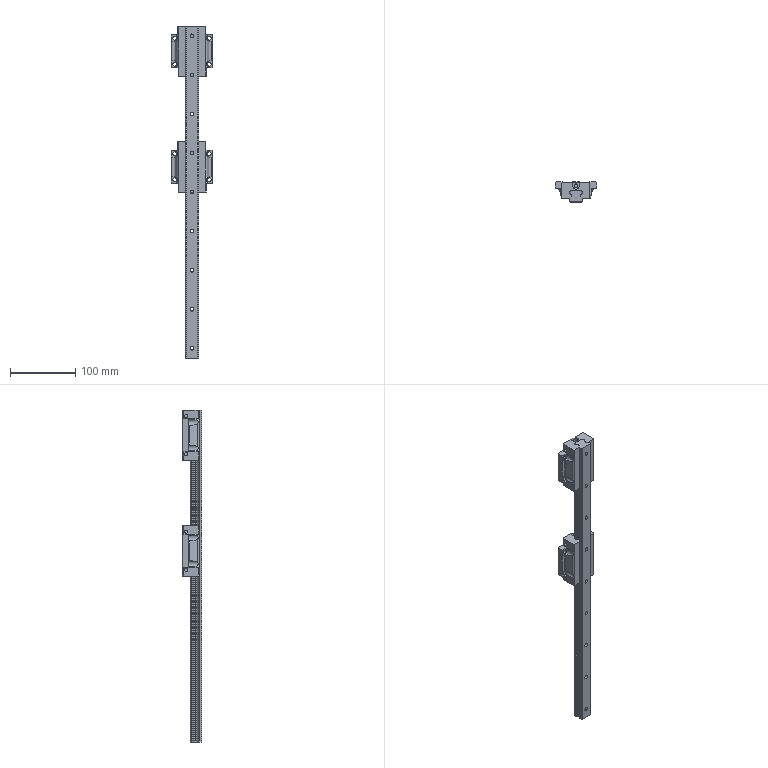Part | SolidWorks | 3 solids | 421 faces | box 63 x 30 x 510 mm | volume 298717 mm3 | plane 239 | cylinder 182 | commonest cylinder face diameters 1 x48 6 x30 10 x24 2 x22 5 x16 4.06 x12